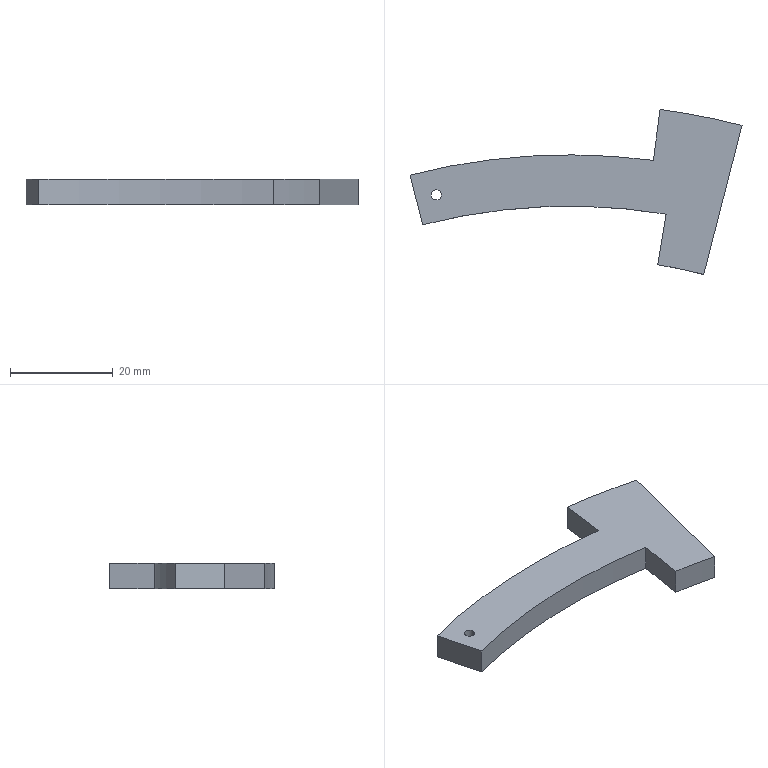Part | SolidWorks | features Extrusion 1, ICE 1 | 1 solid | 12 faces | box 64.703 x 32.148 x 5 mm | volume 4266 mm3 | cylinder 6 | plane 6 | commonest cylinder face diameters 2 x2 210 x1 230 x1 250 x1 270 x1
STEP:
#1=CARTESIAN_POINT('',(-26.989,117.22,5.));
#2=VERTEX_POINT('',#1);
#3=CARTESIAN_POINT('',(-24.989,117.22,5.));
#4=VERTEX_POINT('',#3);
#5=CARTESIAN_POINT('',(-25.989,117.22,5.));
#6=DIRECTION('',(0.,0.,1.));
#7=DIRECTION('',(1.,0.,0.));
#8=AXIS2_PLACEMENT_3D('',#5,#6,#7);
#9=CIRCLE('',#8,1.);
#10=EDGE_CURVE('',#2,#4,#9,.T.);
#11=ORIENTED_EDGE('',*,*,#10,.T.);
#12=CARTESIAN_POINT('',(-24.989,117.22,0.));
#13=VERTEX_POINT('',#12);
#14=CARTESIAN_POINT('',(-24.989,117.22,10.));
#15=DIRECTION('',(0.,0.,-1.));
#16=VECTOR('',#15,1000.);
#17=LINE('',#14,#16);
#18=EDGE_CURVE('',#4,#13,#17,.T.);
#19=ORIENTED_EDGE('',*,*,#18,.T.);
#20=CARTESIAN_POINT('',(-26.989,117.22,0.));
#21=VERTEX_POINT('',#20);
#22=CARTESIAN_POINT('',(-25.989,117.22,0.));
#23=DIRECTION('',(0.,0.,-1.));
#24=DIRECTION('',(-1.,0.,0.));
#25=AXIS2_PLACEMENT_3D('',#22,#23,#24);
#26=CIRCLE('',#25,1.);
#27=EDGE_CURVE('',#13,#21,#26,.T.);
#28=ORIENTED_EDGE('',*,*,#27,.T.);
#29=CARTESIAN_POINT('',(-26.989,117.22,10.));
#30=DIRECTION('',(0.,0.,-1.));
#31=VECTOR('',#30,1000.);
#32=LINE('',#29,#31);
#33=EDGE_CURVE('',#2,#21,#32,.T.);
#34=ORIENTED_EDGE('',*,*,#33,.F.);
#35=EDGE_LOOP('',(#11,#19,#28,#34));
#36=FACE_OUTER_BOUND('',#35,.T.);
#37=CARTESIAN_POINT('',(-25.989,117.22,10.));
#38=DIRECTION('',(0.,0.,-1.));
#39=DIRECTION('',(-1.,0.,0.));
#40=AXIS2_PLACEMENT_3D('',#37,#38,#39);
#41=CYLINDRICAL_SURFACE('',#40,1.);
#42=ADVANCED_FACE('',(#36),#41,.F.);
#43=CARTESIAN_POINT('',(17.621,133.845,0.));
#44=VERTEX_POINT('',#43);
#45=CARTESIAN_POINT('',(33.596,130.753,0.));
#46=VERTEX_POINT('',#45);
#47=CARTESIAN_POINT('',(0.,0.,0.));
#48=DIRECTION('',(0.,0.,-1.));
#49=DIRECTION('',(1.,0.,0.));
#50=AXIS2_PLACEMENT_3D('',#47,#48,#49);
#51=CIRCLE('',#50,135.);
#52=EDGE_CURVE('',#44,#46,#51,.T.);
#53=ORIENTED_EDGE('',*,*,#52,.F.);
#54=CARTESIAN_POINT('',(17.621,133.845,5.));
#55=VERTEX_POINT('',#54);
#56=CARTESIAN_POINT('',(17.621,133.845,5.));
#57=DIRECTION('',(0.,0.,-1.));
#58=VECTOR('',#57,1000.);
#59=LINE('',#56,#58);
#60=EDGE_CURVE('',#55,#44,#59,.T.);
#61=ORIENTED_EDGE('',*,*,#60,.F.);
#62=CARTESIAN_POINT('',(33.596,130.753,5.));
#63=VERTEX_POINT('',#62);
#64=CARTESIAN_POINT('',(0.,0.,5.));
#65=DIRECTION('',(0.,0.,-1.));
#66=DIRECTION('',(1.,0.,0.));
#67=AXIS2_PLACEMENT_3D('',#64,#65,#66);
#68=CIRCLE('',#67,135.);
#69=EDGE_CURVE('',#55,#63,#68,.T.);
#70=ORIENTED_EDGE('',*,*,#69,.T.);
#71=CARTESIAN_POINT('',(33.596,130.753,5.));
#72=DIRECTION('',(0.,0.,-1.));
#73=VECTOR('',#72,1000.);
#74=LINE('',#71,#73);
#75=EDGE_CURVE('',#63,#46,#74,.T.);
#76=ORIENTED_EDGE('',*,*,#75,.T.);
#77=EDGE_LOOP('',(#53,#61,#70,#76));
#78=FACE_OUTER_BOUND('',#77,.T.);
#79=CARTESIAN_POINT('',(0.,0.,5.));
#80=DIRECTION('',(0.,0.,-1.));
#81=DIRECTION('',(-1.,0.,0.));
#82=AXIS2_PLACEMENT_3D('',#79,#80,#81);
#83=CYLINDRICAL_SURFACE('',#82,135.);
#84=ADVANCED_FACE('',(#78),#83,.T.);
#85=CARTESIAN_POINT('',(16.316,123.931,0.));
#86=VERTEX_POINT('',#85);
#87=CARTESIAN_POINT('',(0.,0.,0.));
#88=DIRECTION('',(0.1305,0.9914,0.));
#89=VECTOR('',#88,1000.);
#90=LINE('',#87,#89);
#91=EDGE_CURVE('',#86,#44,#90,.T.);
#92=ORIENTED_EDGE('',*,*,#91,.F.);
#93=CARTESIAN_POINT('',(16.316,123.931,5.));
#94=VERTEX_POINT('',#93);
#95=CARTESIAN_POINT('',(16.316,123.931,5.));
#96=DIRECTION('',(0.,0.,-1.));
#97=VECTOR('',#96,1000.);
#98=LINE('',#95,#97);
#99=EDGE_CURVE('',#94,#86,#98,.T.);
#100=ORIENTED_EDGE('',*,*,#99,.F.);
#101=CARTESIAN_POINT('',(0.,0.,5.));
#102=DIRECTION('',(0.1305,0.9914,0.));
#103=VECTOR('',#102,1000.);
#104=LINE('',#101,#103);
#105=EDGE_CURVE('',#94,#55,#104,.T.);
#106=ORIENTED_EDGE('',*,*,#105,.T.);
#107=ORIENTED_EDGE('',*,*,#60,.T.);
#108=EDGE_LOOP('',(#92,#100,#106,#107));
#109=FACE_OUTER_BOUND('',#108,.T.);
#110=CARTESIAN_POINT('',(0.,0.,5.));
#111=DIRECTION('',(-0.9914,0.1305,0.));
#112=DIRECTION('',(-0.1305,-0.9914,0.));
#113=AXIS2_PLACEMENT_3D('',#110,#111,#112);
#114=PLANE('',#113);
#115=ADVANCED_FACE('',(#109),#114,.T.);
#116=CARTESIAN_POINT('',(-31.107,121.067,0.));
#117=VERTEX_POINT('',#116);
#118=CARTESIAN_POINT('',(0.,0.,0.));
#119=DIRECTION('',(0.,0.,1.));
#120=DIRECTION('',(1.,0.,0.));
#121=AXIS2_PLACEMENT_3D('',#118,#119,#120);
#122=CIRCLE('',#121,125.);
#123=EDGE_CURVE('',#86,#117,#122,.T.);
#124=ORIENTED_EDGE('',*,*,#123,.T.);
#125=CARTESIAN_POINT('',(-31.107,121.067,5.));
#126=VERTEX_POINT('',#125);
#127=CARTESIAN_POINT('',(-31.107,121.067,5.));
#128=DIRECTION('',(0.,0.,-1.));
#129=VECTOR('',#128,1000.);
#130=LINE('',#127,#129);
#131=EDGE_CURVE('',#126,#117,#130,.T.);
#132=ORIENTED_EDGE('',*,*,#131,.F.);
#133=CARTESIAN_POINT('',(0.,0.,5.));
#134=DIRECTION('',(0.,0.,1.));
#135=DIRECTION('',(1.,0.,0.));
#136=AXIS2_PLACEMENT_3D('',#133,#134,#135);
#137=CIRCLE('',#136,125.);
#138=EDGE_CURVE('',#94,#126,#137,.T.);
#139=ORIENTED_EDGE('',*,*,#138,.F.);
#140=ORIENTED_EDGE('',*,*,#99,.T.);
#141=EDGE_LOOP('',(#124,#132,#139,#140));
#142=FACE_OUTER_BOUND('',#141,.T.);
#143=CARTESIAN_POINT('',(0.,0.,5.));
#144=DIRECTION('',(0.,0.,-1.));
#145=DIRECTION('',(-1.,0.,0.));
#146=AXIS2_PLACEMENT_3D('',#143,#144,#145);
#147=CYLINDRICAL_SURFACE('',#146,125.);
#148=ADVANCED_FACE('',(#142),#147,.T.);
#149=CARTESIAN_POINT('',(-28.619,111.382,0.));
#150=VERTEX_POINT('',#149);
#151=CARTESIAN_POINT('',(0.,0.,0.));
#152=DIRECTION('',(-0.2489,0.9685,0.));
#153=VECTOR('',#152,1000.);
#154=LINE('',#151,#153);
#155=EDGE_CURVE('',#150,#117,#154,.T.);
#156=ORIENTED_EDGE('',*,*,#155,.F.);
#157=CARTESIAN_POINT('',(-28.619,111.382,5.));
#158=VERTEX_POINT('',#157);
#159=CARTESIAN_POINT('',(-28.619,111.382,5.));
#160=DIRECTION('',(0.,0.,-1.));
#161=VECTOR('',#160,1000.);
#162=LINE('',#159,#161);
#163=EDGE_CURVE('',#158,#150,#162,.T.);
#164=ORIENTED_EDGE('',*,*,#163,.F.);
#165=CARTESIAN_POINT('',(0.,0.,5.));
#166=DIRECTION('',(-0.2489,0.9685,0.));
#167=VECTOR('',#166,1000.);
#168=LINE('',#165,#167);
#169=EDGE_CURVE('',#158,#126,#168,.T.);
#170=ORIENTED_EDGE('',*,*,#169,.T.);
#171=ORIENTED_EDGE('',*,*,#131,.T.);
#172=EDGE_LOOP('',(#156,#164,#170,#171));
#173=FACE_OUTER_BOUND('',#172,.T.);
#174=CARTESIAN_POINT('',(0.,0.,5.));
#175=DIRECTION('',(-0.9685,-0.2489,0.));
#176=DIRECTION('',(0.2489,-0.9685,0.));
#177=AXIS2_PLACEMENT_3D('',#174,#175,#176);
#178=PLANE('',#177);
#179=ADVANCED_FACE('',(#173),#178,.T.);
#180=CARTESIAN_POINT('',(18.802,113.453,0.));
#181=VERTEX_POINT('',#180);
#182=CARTESIAN_POINT('',(0.,0.,0.));
#183=DIRECTION('',(0.,0.,1.));
#184=DIRECTION('',(1.,0.,0.));
#185=AXIS2_PLACEMENT_3D('',#182,#183,#184);
#186=CIRCLE('',#185,115.);
#187=EDGE_CURVE('',#181,#150,#186,.T.);
#188=ORIENTED_EDGE('',*,*,#187,.F.);
#189=CARTESIAN_POINT('',(18.802,113.453,5.));
#190=VERTEX_POINT('',#189);
#191=CARTESIAN_POINT('',(18.802,113.453,5.));
#192=DIRECTION('',(0.,0.,-1.));
#193=VECTOR('',#192,1000.);
#194=LINE('',#191,#193);
#195=EDGE_CURVE('',#190,#181,#194,.T.);
#196=ORIENTED_EDGE('',*,*,#195,.F.);
#197=CARTESIAN_POINT('',(0.,0.,5.));
#198=DIRECTION('',(0.,0.,1.));
#199=DIRECTION('',(1.,0.,0.));
#200=AXIS2_PLACEMENT_3D('',#197,#198,#199);
#201=CIRCLE('',#200,115.);
#202=EDGE_CURVE('',#190,#158,#201,.T.);
#203=ORIENTED_EDGE('',*,*,#202,.T.);
#204=ORIENTED_EDGE('',*,*,#163,.T.);
#205=EDGE_LOOP('',(#188,#196,#203,#204));
#206=FACE_OUTER_BOUND('',#205,.T.);
#207=CARTESIAN_POINT('',(0.,0.,5.));
#208=DIRECTION('',(0.,0.,-1.));
#209=DIRECTION('',(-1.,0.,0.));
#210=AXIS2_PLACEMENT_3D('',#207,#208,#209);
#211=CYLINDRICAL_SURFACE('',#210,115.);
#212=ADVANCED_FACE('',(#206),#211,.F.);
#213=CARTESIAN_POINT('',(17.167,103.587,0.));
#214=VERTEX_POINT('',#213);
#215=CARTESIAN_POINT('',(0.,0.,0.));
#216=DIRECTION('',(-0.1635,-0.9865,0.));
#217=VECTOR('',#216,1000.);
#218=LINE('',#215,#217);
#219=EDGE_CURVE('',#181,#214,#218,.T.);
#220=ORIENTED_EDGE('',*,*,#219,.T.);
#221=CARTESIAN_POINT('',(17.167,103.587,5.));
#222=VERTEX_POINT('',#221);
#223=CARTESIAN_POINT('',(17.167,103.587,5.));
#224=DIRECTION('',(0.,0.,-1.));
#225=VECTOR('',#224,1000.);
#226=LINE('',#223,#225);
#227=EDGE_CURVE('',#222,#214,#226,.T.);
#228=ORIENTED_EDGE('',*,*,#227,.F.);
#229=CARTESIAN_POINT('',(0.,0.,5.));
#230=DIRECTION('',(-0.1635,-0.9865,0.));
#231=VECTOR('',#230,1000.);
#232=LINE('',#229,#231);
#233=EDGE_CURVE('',#190,#222,#232,.T.);
#234=ORIENTED_EDGE('',*,*,#233,.F.);
#235=ORIENTED_EDGE('',*,*,#195,.T.);
#236=EDGE_LOOP('',(#220,#228,#234,#235));
#237=FACE_OUTER_BOUND('',#236,.T.);
#238=CARTESIAN_POINT('',(0.,0.,5.));
#239=DIRECTION('',(0.9865,-0.1635,0.));
#240=DIRECTION('',(0.1635,0.9865,0.));
#241=AXIS2_PLACEMENT_3D('',#238,#239,#240);
#242=PLANE('',#241);
#243=ADVANCED_FACE('',(#237),#242,.F.);
#244=CARTESIAN_POINT('',(26.13,101.697,0.));
#245=VERTEX_POINT('',#244);
#246=CARTESIAN_POINT('',(0.,0.,0.));
#247=DIRECTION('',(0.,0.,-1.));
#248=DIRECTION('',(1.,0.,0.));
#249=AXIS2_PLACEMENT_3D('',#246,#247,#248);
#250=CIRCLE('',#249,105.);
#251=EDGE_CURVE('',#214,#245,#250,.T.);
#252=ORIENTED_EDGE('',*,*,#251,.T.);
#253=CARTESIAN_POINT('',(26.13,101.697,5.));
#254=VERTEX_POINT('',#253);
#255=CARTESIAN_POINT('',(26.13,101.697,5.));
#256=DIRECTION('',(0.,0.,-1.));
#257=VECTOR('',#256,1000.);
#258=LINE('',#255,#257);
#259=EDGE_CURVE('',#254,#245,#258,.T.);
#260=ORIENTED_EDGE('',*,*,#259,.F.);
#261=CARTESIAN_POINT('',(0.,0.,5.));
#262=DIRECTION('',(0.,0.,-1.));
#263=DIRECTION('',(1.,0.,0.));
#264=AXIS2_PLACEMENT_3D('',#261,#262,#263);
#265=CIRCLE('',#264,105.);
#266=EDGE_CURVE('',#222,#254,#265,.T.);
#267=ORIENTED_EDGE('',*,*,#266,.F.);
#268=ORIENTED_EDGE('',*,*,#227,.T.);
#269=EDGE_LOOP('',(#252,#260,#267,#268));
#270=FACE_OUTER_BOUND('',#269,.T.);
#271=CARTESIAN_POINT('',(0.,0.,5.));
#272=DIRECTION('',(0.,0.,-1.));
#273=DIRECTION('',(-1.,0.,0.));
#274=AXIS2_PLACEMENT_3D('',#271,#272,#273);
#275=CYLINDRICAL_SURFACE('',#274,105.);
#276=ADVANCED_FACE('',(#270),#275,.F.);
#277=CARTESIAN_POINT('',(0.,0.,0.));
#278=DIRECTION('',(-0.2489,-0.9685,0.));
#279=VECTOR('',#278,1000.);
#280=LINE('',#277,#279);
#281=EDGE_CURVE('',#46,#245,#280,.T.);
#282=ORIENTED_EDGE('',*,*,#281,.F.);
#283=ORIENTED_EDGE('',*,*,#75,.F.);
#284=CARTESIAN_POINT('',(0.,0.,5.));
#285=DIRECTION('',(-0.2489,-0.9685,0.));
#286=VECTOR('',#285,1000.);
#287=LINE('',#284,#286);
#288=EDGE_CURVE('',#63,#254,#287,.T.);
#289=ORIENTED_EDGE('',*,*,#288,.T.);
#290=ORIENTED_EDGE('',*,*,#259,.T.);
#291=EDGE_LOOP('',(#282,#283,#289,#290));
#292=FACE_OUTER_BOUND('',#291,.T.);
#293=CARTESIAN_POINT('',(0.,0.,5.));
#294=DIRECTION('',(0.9685,-0.2489,0.));
#295=DIRECTION('',(0.2489,0.9685,0.));
#296=AXIS2_PLACEMENT_3D('',#293,#294,#295);
#297=PLANE('',#296);
#298=ADVANCED_FACE('',(#292),#297,.T.);
#299=ORIENTED_EDGE('',*,*,#10,.F.);
#300=CARTESIAN_POINT('',(-25.989,117.22,5.));
#301=DIRECTION('',(0.,0.,1.));
#302=DIRECTION('',(1.,0.,0.));
#303=AXIS2_PLACEMENT_3D('',#300,#301,#302);
#304=CIRCLE('',#303,1.);
#305=EDGE_CURVE('',#4,#2,#304,.T.);
#306=ORIENTED_EDGE('',*,*,#305,.F.);
#307=EDGE_LOOP('',(#299,#306));
#308=FACE_BOUND('',#307,.T.);
#309=ORIENTED_EDGE('',*,*,#69,.F.);
#310=ORIENTED_EDGE('',*,*,#105,.F.);
#311=ORIENTED_EDGE('',*,*,#138,.T.);
#312=ORIENTED_EDGE('',*,*,#169,.F.);
#313=ORIENTED_EDGE('',*,*,#202,.F.);
#314=ORIENTED_EDGE('',*,*,#233,.T.);
#315=ORIENTED_EDGE('',*,*,#266,.T.);
#316=ORIENTED_EDGE('',*,*,#288,.F.);
#317=EDGE_LOOP('',(#309,#310,#311,#312,#313,#314,#315,#316));
#318=FACE_OUTER_BOUND('',#317,.T.);
#319=CARTESIAN_POINT('',(0.,0.,5.));
#320=DIRECTION('',(0.,0.,1.));
#321=DIRECTION('',(1.,0.,0.));
#322=AXIS2_PLACEMENT_3D('',#319,#320,#321);
#323=PLANE('',#322);
#324=ADVANCED_FACE('',(#308,#318),#323,.T.);
#325=CARTESIAN_POINT('',(-25.989,117.22,0.));
#326=DIRECTION('',(0.,0.,-1.));
#327=DIRECTION('',(-1.,0.,0.));
#328=AXIS2_PLACEMENT_3D('',#325,#326,#327);
#329=CIRCLE('',#328,1.);
#330=EDGE_CURVE('',#21,#13,#329,.T.);
#331=ORIENTED_EDGE('',*,*,#330,.F.);
#332=ORIENTED_EDGE('',*,*,#27,.F.);
#333=EDGE_LOOP('',(#331,#332));
#334=FACE_BOUND('',#333,.T.);
#335=ORIENTED_EDGE('',*,*,#52,.T.);
#336=ORIENTED_EDGE('',*,*,#281,.T.);
#337=ORIENTED_EDGE('',*,*,#251,.F.);
#338=ORIENTED_EDGE('',*,*,#219,.F.);
#339=ORIENTED_EDGE('',*,*,#187,.T.);
#340=ORIENTED_EDGE('',*,*,#155,.T.);
#341=ORIENTED_EDGE('',*,*,#123,.F.);
#342=ORIENTED_EDGE('',*,*,#91,.T.);
#343=EDGE_LOOP('',(#335,#336,#337,#338,#339,#340,#341,#342));
#344=FACE_OUTER_BOUND('',#343,.T.);
#345=CARTESIAN_POINT('',(0.,0.,0.));
#346=DIRECTION('',(0.,0.,1.));
#347=DIRECTION('',(1.,0.,0.));
#348=AXIS2_PLACEMENT_3D('',#345,#346,#347);
#349=PLANE('',#348);
#350=ADVANCED_FACE('',(#334,#344),#349,.F.);
#351=ORIENTED_EDGE('',*,*,#18,.F.);
#352=ORIENTED_EDGE('',*,*,#305,.T.);
#353=ORIENTED_EDGE('',*,*,#33,.T.);
#354=ORIENTED_EDGE('',*,*,#330,.T.);
#355=EDGE_LOOP('',(#351,#352,#353,#354));
#356=FACE_OUTER_BOUND('',#355,.T.);
#357=CARTESIAN_POINT('',(-25.989,117.22,10.));
#358=DIRECTION('',(0.,0.,-1.));
#359=DIRECTION('',(-1.,0.,0.));
#360=AXIS2_PLACEMENT_3D('',#357,#358,#359);
#361=CYLINDRICAL_SURFACE('',#360,1.);
#362=ADVANCED_FACE('',(#356),#361,.F.);
#363=CLOSED_SHELL('',(#42,#84,#115,#148,#179,#212,#243,#276,#298,#324,#350,#362));
#364=MANIFOLD_SOLID_BREP('',#363);
#365=CARTESIAN_POINT('',(0.,0.,0.));
#366=DIRECTION('',(0.,0.,1.));
#367=DIRECTION('',(1.,0.,0.));
#368=AXIS2_PLACEMENT_3D('',#365,#366,#367);
#369=(LENGTH_UNIT()NAMED_UNIT(*)SI_UNIT(.MILLI.,.METRE.));
#370=UNCERTAINTY_MEASURE_WITH_UNIT(LENGTH_MEASURE(0.00001),#369,'','');
#371=(NAMED_UNIT(*)PLANE_ANGLE_UNIT()SI_UNIT($,.RADIAN.));
#372=(NAMED_UNIT(*)SI_UNIT($,.STERADIAN.)SOLID_ANGLE_UNIT());
#373=(GEOMETRIC_REPRESENTATION_CONTEXT(3)GLOBAL_UNCERTAINTY_ASSIGNED_CONTEXT((#370))GLOBAL_UNIT_ASSIGNED_CONTEXT((#369,#371,#372))REPRESENTATION_CONTEXT('',''));
#374=ADVANCED_BREP_SHAPE_REPRESENTATION('',(#364,#368),#373);